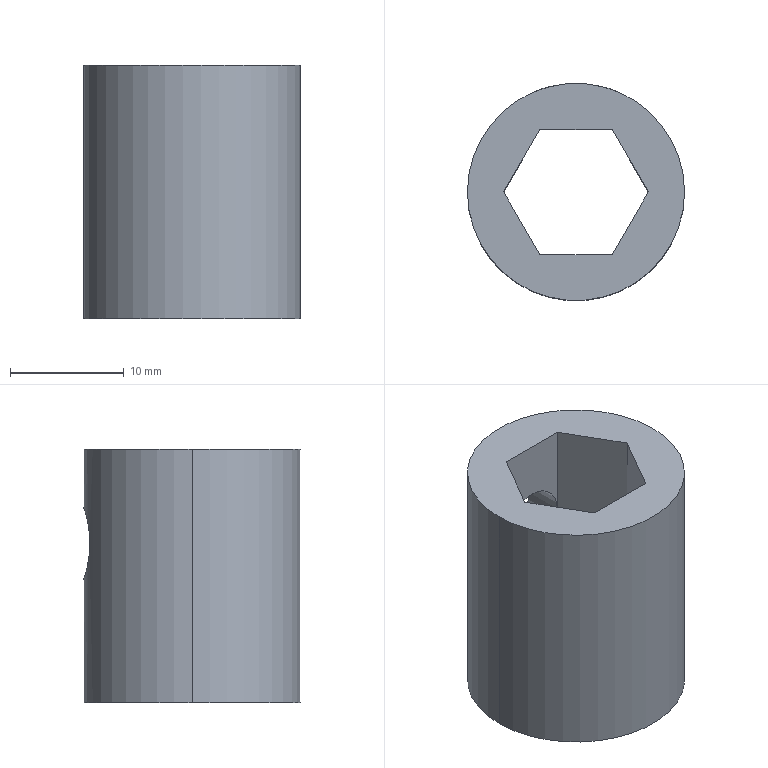Part | NX | features BREP 1 | 1 solid | 13 faces | box 19.05 x 19.05 x 22.225 mm | volume 3883 mm3 | plane 9 | cylinder 4 | commonest cylinder face diameters 6.35 x2 19.05 x2
STEP:
#1=CARTESIAN_POINT('',(-9.525,0.,0.));
#2=VERTEX_POINT('',#1);
#3=CARTESIAN_POINT('',(9.525,0.,0.));
#4=VERTEX_POINT('',#3);
#5=CARTESIAN_POINT('',(0.,0.,0.));
#6=DIRECTION('',(0.,0.,1.));
#7=DIRECTION('',(-1.,0.,0.));
#8=AXIS2_PLACEMENT_3D('',#5,#6,#7);
#9=CIRCLE('',#8,9.525);
#10=EDGE_CURVE('',#2,#4,#9,.T.);
#11=ORIENTED_EDGE('',*,*,#10,.F.);
#12=CARTESIAN_POINT('',(0.,0.,0.));
#13=DIRECTION('',(0.,0.,1.));
#14=DIRECTION('',(1.,0.,0.));
#15=AXIS2_PLACEMENT_3D('',#12,#13,#14);
#16=CIRCLE('',#15,9.525);
#17=EDGE_CURVE('',#4,#2,#16,.T.);
#18=ORIENTED_EDGE('',*,*,#17,.F.);
#19=EDGE_LOOP('',(#11,#18));
#20=FACE_BOUND('',#19,.T.);
#21=CARTESIAN_POINT('',(3.175,-5.499,0.));
#22=VERTEX_POINT('',#21);
#23=CARTESIAN_POINT('',(-3.175,-5.499,0.));
#24=VERTEX_POINT('',#23);
#25=CARTESIAN_POINT('',(3.175,-5.499,0.));
#26=DIRECTION('',(-1.,0.,0.));
#27=VECTOR('',#26,1000.);
#28=LINE('',#25,#27);
#29=EDGE_CURVE('',#22,#24,#28,.T.);
#30=ORIENTED_EDGE('',*,*,#29,.F.);
#31=CARTESIAN_POINT('',(6.35,0.,0.));
#32=VERTEX_POINT('',#31);
#33=CARTESIAN_POINT('',(6.35,0.,0.));
#34=DIRECTION('',(-0.5,-0.866,0.));
#35=VECTOR('',#34,1000.);
#36=LINE('',#33,#35);
#37=EDGE_CURVE('',#32,#22,#36,.T.);
#38=ORIENTED_EDGE('',*,*,#37,.F.);
#39=CARTESIAN_POINT('',(3.175,5.499,0.));
#40=VERTEX_POINT('',#39);
#41=CARTESIAN_POINT('',(3.175,5.499,0.));
#42=DIRECTION('',(0.5,-0.866,0.));
#43=VECTOR('',#42,1000.);
#44=LINE('',#41,#43);
#45=EDGE_CURVE('',#40,#32,#44,.T.);
#46=ORIENTED_EDGE('',*,*,#45,.F.);
#47=CARTESIAN_POINT('',(-3.175,5.499,0.));
#48=VERTEX_POINT('',#47);
#49=CARTESIAN_POINT('',(-3.175,5.499,0.));
#50=DIRECTION('',(1.,0.,0.));
#51=VECTOR('',#50,1000.);
#52=LINE('',#49,#51);
#53=EDGE_CURVE('',#48,#40,#52,.T.);
#54=ORIENTED_EDGE('',*,*,#53,.F.);
#55=CARTESIAN_POINT('',(-6.35,0.,0.));
#56=VERTEX_POINT('',#55);
#57=CARTESIAN_POINT('',(-6.35,0.,0.));
#58=DIRECTION('',(0.5,0.866,0.));
#59=VECTOR('',#58,1000.);
#60=LINE('',#57,#59);
#61=EDGE_CURVE('',#56,#48,#60,.T.);
#62=ORIENTED_EDGE('',*,*,#61,.F.);
#63=CARTESIAN_POINT('',(-3.175,-5.499,0.));
#64=DIRECTION('',(-0.5,0.866,0.));
#65=VECTOR('',#64,1000.);
#66=LINE('',#63,#65);
#67=EDGE_CURVE('',#24,#56,#66,.T.);
#68=ORIENTED_EDGE('',*,*,#67,.F.);
#69=EDGE_LOOP('',(#30,#38,#46,#54,#62,#68));
#70=FACE_BOUND('',#69,.T.);
#71=CARTESIAN_POINT('',(0.,0.,0.));
#72=DIRECTION('',(0.,0.,1.));
#73=DIRECTION('',(1.,0.,0.));
#74=AXIS2_PLACEMENT_3D('',#71,#72,#73);
#75=PLANE('',#74);
#76=ADVANCED_FACE('',(#20,#70),#75,.F.);
#77=CARTESIAN_POINT('',(-9.525,0.,22.225));
#78=VERTEX_POINT('',#77);
#79=CARTESIAN_POINT('',(-9.525,0.,0.));
#80=DIRECTION('',(0.,0.,1.));
#81=VECTOR('',#80,1000.);
#82=LINE('',#79,#81);
#83=EDGE_CURVE('',#2,#78,#82,.T.);
#84=ORIENTED_EDGE('',*,*,#83,.T.);
#85=CARTESIAN_POINT('',(9.525,0.,22.225));
#86=VERTEX_POINT('',#85);
#87=CARTESIAN_POINT('',(0.,0.,22.225));
#88=DIRECTION('',(0.,0.,1.));
#89=DIRECTION('',(1.,0.,0.));
#90=AXIS2_PLACEMENT_3D('',#87,#88,#89);
#91=CIRCLE('',#90,9.525);
#92=EDGE_CURVE('',#86,#78,#91,.T.);
#93=ORIENTED_EDGE('',*,*,#92,.F.);
#94=CARTESIAN_POINT('',(9.525,0.,0.));
#95=DIRECTION('',(0.,0.,1.));
#96=VECTOR('',#95,1000.);
#97=LINE('',#94,#96);
#98=EDGE_CURVE('',#4,#86,#97,.T.);
#99=ORIENTED_EDGE('',*,*,#98,.F.);
#100=ORIENTED_EDGE('',*,*,#17,.T.);
#101=EDGE_LOOP('',(#84,#93,#99,#100));
#102=FACE_BOUND('',#101,.T.);
#103=CARTESIAN_POINT('',(0.,9.525,10.795));
#104=VERTEX_POINT('',#103);
#105=CARTESIAN_POINT('',(0.,9.525,17.145));
#106=VERTEX_POINT('',#105);
#107=CARTESIAN_POINT('',(0.,9.525,10.795));
#108=CARTESIAN_POINT('',(0.8311,9.525,10.795));
#109=CARTESIAN_POINT('',(2.491,9.26,11.485));
#110=CARTESIAN_POINT('',(3.517,8.84,13.97));
#111=CARTESIAN_POINT('',(2.491,9.26,16.455));
#112=CARTESIAN_POINT('',(0.8314,9.525,17.145));
#113=CARTESIAN_POINT('',(0.,9.525,17.145));
#114=B_SPLINE_CURVE_WITH_KNOTS('',3,(#107,#108,#109,#110,#111,#112,#113),.UNSPECIFIED.,.F.,.F.,(4,1,1,1,4),(0.,0.25,0.5,0.75,1.),.UNSPECIFIED.);
#115=EDGE_CURVE('',#104,#106,#114,.T.);
#116=ORIENTED_EDGE('',*,*,#115,.T.);
#117=CARTESIAN_POINT('',(0.,9.525,17.145));
#118=CARTESIAN_POINT('',(-0.8311,9.525,17.145));
#119=CARTESIAN_POINT('',(-2.491,9.26,16.455));
#120=CARTESIAN_POINT('',(-3.517,8.84,13.97));
#121=CARTESIAN_POINT('',(-2.49,9.26,11.485));
#122=CARTESIAN_POINT('',(-0.8313,9.525,10.795));
#123=CARTESIAN_POINT('',(0.,9.525,10.795));
#124=B_SPLINE_CURVE_WITH_KNOTS('',3,(#117,#118,#119,#120,#121,#122,#123),.UNSPECIFIED.,.F.,.F.,(4,1,1,1,4),(0.,0.25,0.5,0.75,1.),.UNSPECIFIED.);
#125=EDGE_CURVE('',#106,#104,#124,.T.);
#126=ORIENTED_EDGE('',*,*,#125,.T.);
#127=EDGE_LOOP('',(#116,#126));
#128=FACE_BOUND('',#127,.T.);
#129=CARTESIAN_POINT('',(0.,0.,0.));
#130=DIRECTION('',(0.,0.,1.));
#131=DIRECTION('',(1.,0.,0.));
#132=AXIS2_PLACEMENT_3D('',#129,#130,#131);
#133=CYLINDRICAL_SURFACE('',#132,9.525);
#134=ADVANCED_FACE('',(#102,#128),#133,.T.);
#135=ORIENTED_EDGE('',*,*,#98,.T.);
#136=CARTESIAN_POINT('',(0.,0.,22.225));
#137=DIRECTION('',(0.,0.,1.));
#138=DIRECTION('',(-1.,0.,0.));
#139=AXIS2_PLACEMENT_3D('',#136,#137,#138);
#140=CIRCLE('',#139,9.525);
#141=EDGE_CURVE('',#78,#86,#140,.T.);
#142=ORIENTED_EDGE('',*,*,#141,.F.);
#143=ORIENTED_EDGE('',*,*,#83,.F.);
#144=ORIENTED_EDGE('',*,*,#10,.T.);
#145=EDGE_LOOP('',(#135,#142,#143,#144));
#146=FACE_BOUND('',#145,.T.);
#147=CARTESIAN_POINT('',(0.,0.,0.));
#148=DIRECTION('',(0.,0.,1.));
#149=DIRECTION('',(1.,0.,0.));
#150=AXIS2_PLACEMENT_3D('',#147,#148,#149);
#151=CYLINDRICAL_SURFACE('',#150,9.525);
#152=ADVANCED_FACE('',(#146),#151,.T.);
#153=ORIENTED_EDGE('',*,*,#141,.T.);
#154=ORIENTED_EDGE('',*,*,#92,.T.);
#155=EDGE_LOOP('',(#153,#154));
#156=FACE_BOUND('',#155,.T.);
#157=CARTESIAN_POINT('',(-6.35,0.,22.225));
#158=VERTEX_POINT('',#157);
#159=CARTESIAN_POINT('',(-3.175,5.499,22.225));
#160=VERTEX_POINT('',#159);
#161=CARTESIAN_POINT('',(-6.35,0.,22.225));
#162=DIRECTION('',(0.5,0.866,0.));
#163=VECTOR('',#162,1000.);
#164=LINE('',#161,#163);
#165=EDGE_CURVE('',#158,#160,#164,.T.);
#166=ORIENTED_EDGE('',*,*,#165,.T.);
#167=CARTESIAN_POINT('',(3.175,5.499,22.225));
#168=VERTEX_POINT('',#167);
#169=CARTESIAN_POINT('',(-3.175,5.499,22.225));
#170=DIRECTION('',(1.,0.,0.));
#171=VECTOR('',#170,1000.);
#172=LINE('',#169,#171);
#173=EDGE_CURVE('',#160,#168,#172,.T.);
#174=ORIENTED_EDGE('',*,*,#173,.T.);
#175=CARTESIAN_POINT('',(6.35,0.,22.225));
#176=VERTEX_POINT('',#175);
#177=CARTESIAN_POINT('',(3.175,5.499,22.225));
#178=DIRECTION('',(0.5,-0.866,0.));
#179=VECTOR('',#178,1000.);
#180=LINE('',#177,#179);
#181=EDGE_CURVE('',#168,#176,#180,.T.);
#182=ORIENTED_EDGE('',*,*,#181,.T.);
#183=CARTESIAN_POINT('',(3.175,-5.499,22.225));
#184=VERTEX_POINT('',#183);
#185=CARTESIAN_POINT('',(6.35,0.,22.225));
#186=DIRECTION('',(-0.5,-0.866,0.));
#187=VECTOR('',#186,1000.);
#188=LINE('',#185,#187);
#189=EDGE_CURVE('',#176,#184,#188,.T.);
#190=ORIENTED_EDGE('',*,*,#189,.T.);
#191=CARTESIAN_POINT('',(-3.175,-5.499,22.225));
#192=VERTEX_POINT('',#191);
#193=CARTESIAN_POINT('',(3.175,-5.499,22.225));
#194=DIRECTION('',(-1.,0.,0.));
#195=VECTOR('',#194,1000.);
#196=LINE('',#193,#195);
#197=EDGE_CURVE('',#184,#192,#196,.T.);
#198=ORIENTED_EDGE('',*,*,#197,.T.);
#199=CARTESIAN_POINT('',(-3.175,-5.499,22.225));
#200=DIRECTION('',(-0.5,0.866,0.));
#201=VECTOR('',#200,1000.);
#202=LINE('',#199,#201);
#203=EDGE_CURVE('',#192,#158,#202,.T.);
#204=ORIENTED_EDGE('',*,*,#203,.T.);
#205=EDGE_LOOP('',(#166,#174,#182,#190,#198,#204));
#206=FACE_BOUND('',#205,.T.);
#207=CARTESIAN_POINT('',(0.,0.,22.225));
#208=DIRECTION('',(0.,0.,1.));
#209=DIRECTION('',(1.,0.,0.));
#210=AXIS2_PLACEMENT_3D('',#207,#208,#209);
#211=PLANE('',#210);
#212=ADVANCED_FACE('',(#156,#206),#211,.T.);
#213=CARTESIAN_POINT('',(-6.35,0.,0.));
#214=DIRECTION('',(0.,0.,1.));
#215=VECTOR('',#214,1000.);
#216=LINE('',#213,#215);
#217=EDGE_CURVE('',#56,#158,#216,.T.);
#218=ORIENTED_EDGE('',*,*,#217,.T.);
#219=ORIENTED_EDGE('',*,*,#203,.F.);
#220=CARTESIAN_POINT('',(-3.175,-5.499,0.));
#221=DIRECTION('',(0.,0.,1.));
#222=VECTOR('',#221,1000.);
#223=LINE('',#220,#222);
#224=EDGE_CURVE('',#24,#192,#223,.T.);
#225=ORIENTED_EDGE('',*,*,#224,.F.);
#226=ORIENTED_EDGE('',*,*,#67,.T.);
#227=EDGE_LOOP('',(#218,#219,#225,#226));
#228=FACE_BOUND('',#227,.T.);
#229=CARTESIAN_POINT('',(-3.175,-5.499,0.));
#230=DIRECTION('',(-0.866,-0.5,0.));
#231=DIRECTION('',(-0.5,0.866,0.));
#232=AXIS2_PLACEMENT_3D('',#229,#230,#231);
#233=PLANE('',#232);
#234=ADVANCED_FACE('',(#228),#233,.F.);
#235=ORIENTED_EDGE('',*,*,#224,.T.);
#236=ORIENTED_EDGE('',*,*,#197,.F.);
#237=CARTESIAN_POINT('',(3.175,-5.499,0.));
#238=DIRECTION('',(0.,0.,1.));
#239=VECTOR('',#238,1000.);
#240=LINE('',#237,#239);
#241=EDGE_CURVE('',#22,#184,#240,.T.);
#242=ORIENTED_EDGE('',*,*,#241,.F.);
#243=ORIENTED_EDGE('',*,*,#29,.T.);
#244=EDGE_LOOP('',(#235,#236,#242,#243));
#245=FACE_BOUND('',#244,.T.);
#246=CARTESIAN_POINT('',(3.175,-5.499,0.));
#247=DIRECTION('',(0.,-1.,0.));
#248=DIRECTION('',(0.,0.,-1.));
#249=AXIS2_PLACEMENT_3D('',#246,#247,#248);
#250=PLANE('',#249);
#251=ADVANCED_FACE('',(#245),#250,.F.);
#252=ORIENTED_EDGE('',*,*,#241,.T.);
#253=ORIENTED_EDGE('',*,*,#189,.F.);
#254=CARTESIAN_POINT('',(6.35,0.,0.));
#255=DIRECTION('',(0.,0.,1.));
#256=VECTOR('',#255,1000.);
#257=LINE('',#254,#256);
#258=EDGE_CURVE('',#32,#176,#257,.T.);
#259=ORIENTED_EDGE('',*,*,#258,.F.);
#260=ORIENTED_EDGE('',*,*,#37,.T.);
#261=EDGE_LOOP('',(#252,#253,#259,#260));
#262=FACE_BOUND('',#261,.T.);
#263=CARTESIAN_POINT('',(6.35,0.,0.));
#264=DIRECTION('',(0.866,-0.5,0.));
#265=DIRECTION('',(0.,0.,-1.));
#266=AXIS2_PLACEMENT_3D('',#263,#264,#265);
#267=PLANE('',#266);
#268=ADVANCED_FACE('',(#262),#267,.F.);
#269=CARTESIAN_POINT('',(3.175,5.499,13.946));
#270=VERTEX_POINT('',#269);
#271=CARTESIAN_POINT('',(3.175,5.499,0.));
#272=DIRECTION('',(0.,0.,1.));
#273=VECTOR('',#272,1000.);
#274=LINE('',#271,#273);
#275=EDGE_CURVE('',#40,#270,#274,.T.);
#276=ORIENTED_EDGE('',*,*,#275,.F.);
#277=ORIENTED_EDGE('',*,*,#45,.T.);
#278=ORIENTED_EDGE('',*,*,#258,.T.);
#279=ORIENTED_EDGE('',*,*,#181,.F.);
#280=CARTESIAN_POINT('',(3.175,5.499,13.994));
#281=VERTEX_POINT('',#280);
#282=CARTESIAN_POINT('',(3.175,5.499,13.994));
#283=DIRECTION('',(0.,0.,1.));
#284=VECTOR('',#283,1000.);
#285=LINE('',#282,#284);
#286=EDGE_CURVE('',#281,#168,#285,.T.);
#287=ORIENTED_EDGE('',*,*,#286,.F.);
#288=CARTESIAN_POINT('',(3.175,5.499,13.946));
#289=CARTESIAN_POINT('',(3.175,5.499,13.962));
#290=CARTESIAN_POINT('',(3.175,5.499,13.978));
#291=CARTESIAN_POINT('',(3.175,5.499,13.994));
#292=B_SPLINE_CURVE_WITH_KNOTS('',3,(#288,#289,#290,#291),.UNSPECIFIED.,.F.,.F.,(4,4),(0.,1.),.UNSPECIFIED.);
#293=EDGE_CURVE('',#270,#281,#292,.T.);
#294=ORIENTED_EDGE('',*,*,#293,.F.);
#295=EDGE_LOOP('',(#276,#277,#278,#279,#287,#294));
#296=FACE_BOUND('',#295,.T.);
#297=CARTESIAN_POINT('',(3.175,5.499,0.));
#298=DIRECTION('',(0.866,0.5,0.));
#299=DIRECTION('',(0.,0.,-1.));
#300=AXIS2_PLACEMENT_3D('',#297,#298,#299);
#301=PLANE('',#300);
#302=ADVANCED_FACE('',(#296),#301,.F.);
#303=CARTESIAN_POINT('',(0.,5.499,10.795));
#304=VERTEX_POINT('',#303);
#305=CARTESIAN_POINT('',(0.,5.499,10.795));
#306=DIRECTION('',(0.,1.,0.));
#307=VECTOR('',#306,1000.);
#308=LINE('',#305,#307);
#309=EDGE_CURVE('',#304,#104,#308,.T.);
#310=ORIENTED_EDGE('',*,*,#309,.F.);
#311=CARTESIAN_POINT('',(0.,5.499,13.97));
#312=DIRECTION('',(0.,-1.,0.));
#313=DIRECTION('',(0.,0.,-1.));
#314=AXIS2_PLACEMENT_3D('',#311,#312,#313);
#315=CIRCLE('',#314,3.175);
#316=EDGE_CURVE('',#304,#270,#315,.T.);
#317=ORIENTED_EDGE('',*,*,#316,.T.);
#318=ORIENTED_EDGE('',*,*,#293,.T.);
#319=CARTESIAN_POINT('',(0.,5.499,17.145));
#320=VERTEX_POINT('',#319);
#321=CARTESIAN_POINT('',(0.,5.499,13.97));
#322=DIRECTION('',(0.,-1.,0.));
#323=DIRECTION('',(1.,0.,0.007659));
#324=AXIS2_PLACEMENT_3D('',#321,#322,#323);
#325=CIRCLE('',#324,3.175);
#326=EDGE_CURVE('',#281,#320,#325,.T.);
#327=ORIENTED_EDGE('',*,*,#326,.T.);
#328=CARTESIAN_POINT('',(0.,5.499,17.145));
#329=DIRECTION('',(0.,1.,0.));
#330=VECTOR('',#329,1000.);
#331=LINE('',#328,#330);
#332=EDGE_CURVE('',#320,#106,#331,.T.);
#333=ORIENTED_EDGE('',*,*,#332,.T.);
#334=ORIENTED_EDGE('',*,*,#115,.F.);
#335=EDGE_LOOP('',(#310,#317,#318,#327,#333,#334));
#336=FACE_BOUND('',#335,.T.);
#337=CARTESIAN_POINT('',(0.,5.499,13.97));
#338=DIRECTION('',(0.,-1.,0.));
#339=DIRECTION('',(0.,0.,1.));
#340=AXIS2_PLACEMENT_3D('',#337,#338,#339);
#341=CYLINDRICAL_SURFACE('',#340,3.175);
#342=ADVANCED_FACE('',(#336),#341,.F.);
#343=ORIENTED_EDGE('',*,*,#332,.F.);
#344=CARTESIAN_POINT('',(-3.175,5.499,13.994));
#345=VERTEX_POINT('',#344);
#346=CARTESIAN_POINT('',(0.,5.499,13.97));
#347=DIRECTION('',(0.,-1.,0.));
#348=DIRECTION('',(0.,0.,1.));
#349=AXIS2_PLACEMENT_3D('',#346,#347,#348);
#350=CIRCLE('',#349,3.175);
#351=EDGE_CURVE('',#320,#345,#350,.T.);
#352=ORIENTED_EDGE('',*,*,#351,.T.);
#353=CARTESIAN_POINT('',(-3.175,5.499,13.946));
#354=VERTEX_POINT('',#353);
#355=CARTESIAN_POINT('',(-3.175,5.499,13.946));
#356=CARTESIAN_POINT('',(-3.175,5.499,13.962));
#357=CARTESIAN_POINT('',(-3.175,5.499,13.978));
#358=CARTESIAN_POINT('',(-3.175,5.499,13.994));
#359=B_SPLINE_CURVE_WITH_KNOTS('',3,(#355,#356,#357,#358),.UNSPECIFIED.,.F.,.F.,(4,4),(0.,1.),.UNSPECIFIED.);
#360=EDGE_CURVE('',#354,#345,#359,.T.);
#361=ORIENTED_EDGE('',*,*,#360,.F.);
#362=CARTESIAN_POINT('',(0.,5.499,13.97));
#363=DIRECTION('',(0.,-1.,0.));
#364=DIRECTION('',(-1.,0.,-0.007659));
#365=AXIS2_PLACEMENT_3D('',#362,#363,#364);
#366=CIRCLE('',#365,3.175);
#367=EDGE_CURVE('',#354,#304,#366,.T.);
#368=ORIENTED_EDGE('',*,*,#367,.T.);
#369=ORIENTED_EDGE('',*,*,#309,.T.);
#370=ORIENTED_EDGE('',*,*,#125,.F.);
#371=EDGE_LOOP('',(#343,#352,#361,#368,#369,#370));
#372=FACE_BOUND('',#371,.T.);
#373=CARTESIAN_POINT('',(0.,5.499,13.97));
#374=DIRECTION('',(0.,-1.,0.));
#375=DIRECTION('',(0.,0.,1.));
#376=AXIS2_PLACEMENT_3D('',#373,#374,#375);
#377=CYLINDRICAL_SURFACE('',#376,3.175);
#378=ADVANCED_FACE('',(#372),#377,.F.);
#379=ORIENTED_EDGE('',*,*,#326,.F.);
#380=ORIENTED_EDGE('',*,*,#286,.T.);
#381=ORIENTED_EDGE('',*,*,#173,.F.);
#382=CARTESIAN_POINT('',(-3.175,5.499,13.994));
#383=DIRECTION('',(0.,0.,1.));
#384=VECTOR('',#383,1000.);
#385=LINE('',#382,#384);
#386=EDGE_CURVE('',#345,#160,#385,.T.);
#387=ORIENTED_EDGE('',*,*,#386,.F.);
#388=ORIENTED_EDGE('',*,*,#351,.F.);
#389=EDGE_LOOP('',(#379,#380,#381,#387,#388));
#390=FACE_BOUND('',#389,.T.);
#391=CARTESIAN_POINT('',(-3.175,5.499,0.));
#392=DIRECTION('',(0.,1.,0.));
#393=DIRECTION('',(1.,0.,0.));
#394=AXIS2_PLACEMENT_3D('',#391,#392,#393);
#395=PLANE('',#394);
#396=ADVANCED_FACE('',(#390),#395,.F.);
#397=ORIENTED_EDGE('',*,*,#367,.F.);
#398=CARTESIAN_POINT('',(-3.175,5.499,0.));
#399=DIRECTION('',(0.,0.,1.));
#400=VECTOR('',#399,1000.);
#401=LINE('',#398,#400);
#402=EDGE_CURVE('',#48,#354,#401,.T.);
#403=ORIENTED_EDGE('',*,*,#402,.F.);
#404=ORIENTED_EDGE('',*,*,#53,.T.);
#405=ORIENTED_EDGE('',*,*,#275,.T.);
#406=ORIENTED_EDGE('',*,*,#316,.F.);
#407=EDGE_LOOP('',(#397,#403,#404,#405,#406));
#408=FACE_BOUND('',#407,.T.);
#409=CARTESIAN_POINT('',(-3.175,5.499,0.));
#410=DIRECTION('',(0.,1.,0.));
#411=DIRECTION('',(1.,0.,0.));
#412=AXIS2_PLACEMENT_3D('',#409,#410,#411);
#413=PLANE('',#412);
#414=ADVANCED_FACE('',(#408),#413,.F.);
#415=ORIENTED_EDGE('',*,*,#386,.T.);
#416=ORIENTED_EDGE('',*,*,#165,.F.);
#417=ORIENTED_EDGE('',*,*,#217,.F.);
#418=ORIENTED_EDGE('',*,*,#61,.T.);
#419=ORIENTED_EDGE('',*,*,#402,.T.);
#420=ORIENTED_EDGE('',*,*,#360,.T.);
#421=EDGE_LOOP('',(#415,#416,#417,#418,#419,#420));
#422=FACE_BOUND('',#421,.T.);
#423=CARTESIAN_POINT('',(-6.35,0.,0.));
#424=DIRECTION('',(-0.866,0.5,0.));
#425=DIRECTION('',(0.,0.,1.));
#426=AXIS2_PLACEMENT_3D('',#423,#424,#425);
#427=PLANE('',#426);
#428=ADVANCED_FACE('',(#422),#427,.F.);
#429=CLOSED_SHELL('',(#76,#134,#152,#212,#234,#251,#268,#302,#342,#378,#396,#414,#428));
#430=MANIFOLD_SOLID_BREP('',#429);
#431=(LENGTH_UNIT()NAMED_UNIT(*)SI_UNIT(.MILLI.,.METRE.));
#432=UNCERTAINTY_MEASURE_WITH_UNIT(LENGTH_MEASURE(0.0508),#431,'','');
#433=(NAMED_UNIT(*)PLANE_ANGLE_UNIT()SI_UNIT($,.RADIAN.));
#434=(NAMED_UNIT(*)SI_UNIT($,.STERADIAN.)SOLID_ANGLE_UNIT());
#435=(GEOMETRIC_REPRESENTATION_CONTEXT(3)GLOBAL_UNCERTAINTY_ASSIGNED_CONTEXT((#432))GLOBAL_UNIT_ASSIGNED_CONTEXT((#431,#433,#434))REPRESENTATION_CONTEXT('',''));
#436=ADVANCED_BREP_SHAPE_REPRESENTATION('',(#430),#435);